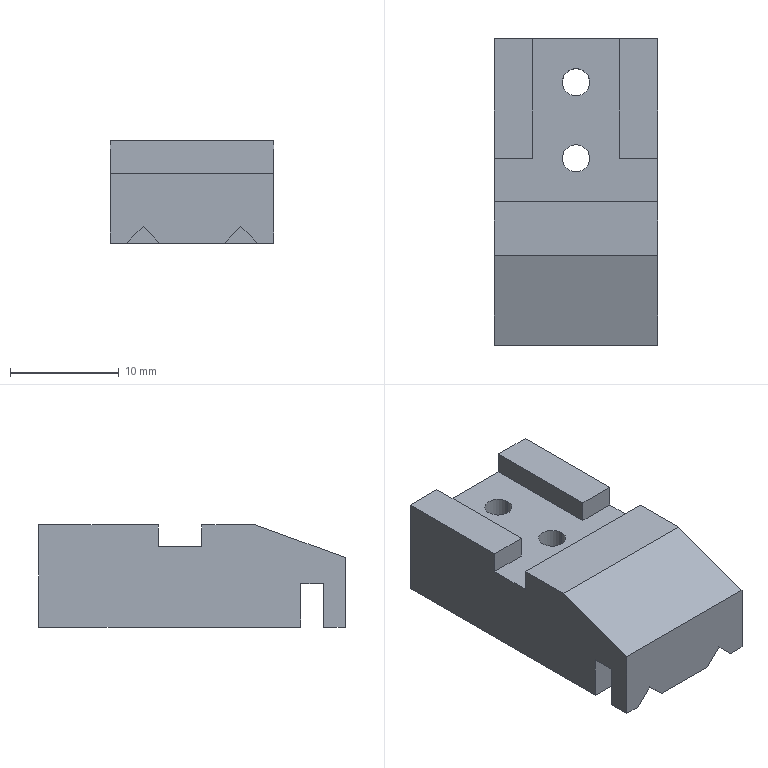Part | STEP file | A05 | 1 solid | 29 faces | box 15 x 28.2 x 9.4 mm | volume 3287 mm3 | plane 25 | cylinder 4 | commonest cylinder face diameters 2.5 x4